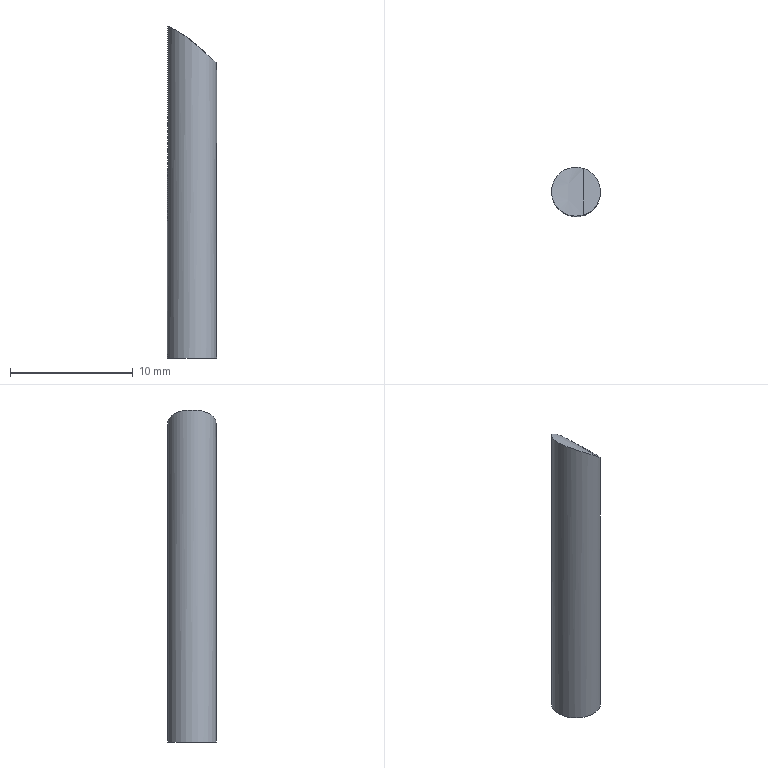Part | NX | features solid 2 | 1 solid | 4 faces | box 4 x 4.001 x 27.078 mm | volume 323.75 mm3 | spline 2 | cylinder 1 | plane 1 | commonest cylinder face diameters 4 x1
STEP:
#1=CARTESIAN_POINT('',(870.5,-198.,17.));
#2=VERTEX_POINT('',#1);
#3=CARTESIAN_POINT('',(872.5,-198.,17.));
#4=DIRECTION('',(0.,0.,-1.));
#5=DIRECTION('',(-1.,0.,0.));
#6=AXIS2_PLACEMENT_3D('',#3,#4,#5);
#7=CIRCLE('',#6,2.);
#8=EDGE_CURVE('',#2,#2,#7,.T.);
#9=ORIENTED_EDGE('',*,*,#8,.F.);
#10=EDGE_LOOP('',(#9));
#11=FACE_BOUND('',#10,.T.);
#12=CARTESIAN_POINT('',(873.077,-199.915,42.346));
#13=VERTEX_POINT('',#12);
#14=CARTESIAN_POINT('',(873.122,-196.099,42.33));
#15=VERTEX_POINT('',#14);
#16=CARTESIAN_POINT('',(873.077,-199.915,42.346));
#17=CARTESIAN_POINT('',(873.426,-199.81,42.025));
#18=CARTESIAN_POINT('',(874.098,-199.426,41.407));
#19=CARTESIAN_POINT('',(874.692,-198.034,40.865));
#20=CARTESIAN_POINT('',(874.135,-196.613,41.387));
#21=CARTESIAN_POINT('',(873.469,-196.212,42.007));
#22=CARTESIAN_POINT('',(873.122,-196.099,42.33));
#23=B_SPLINE_CURVE_WITH_KNOTS('',3,(#16,#17,#18,#19,#20,#21,#22),.UNSPECIFIED.,.F.,.F.,(4,1,1,1,4),(0.00009288,0.001538,0.002982,0.004427,0.005872),.UNSPECIFIED.);
#24=EDGE_CURVE('',#13,#15,#23,.T.);
#25=ORIENTED_EDGE('',*,*,#24,.F.);
#26=CARTESIAN_POINT('',(873.077,-199.915,42.346));
#27=CARTESIAN_POINT('',(872.568,-200.068,42.816));
#28=CARTESIAN_POINT('',(871.655,-200.006,43.483));
#29=CARTESIAN_POINT('',(870.685,-199.041,43.992));
#30=CARTESIAN_POINT('',(870.403,-197.978,44.121));
#31=CARTESIAN_POINT('',(870.707,-196.923,43.989));
#32=CARTESIAN_POINT('',(871.699,-195.974,43.474));
#33=CARTESIAN_POINT('',(872.616,-195.934,42.8));
#34=CARTESIAN_POINT('',(873.122,-196.099,42.33));
#35=B_SPLINE_CURVE_WITH_KNOTS('',3,(#26,#27,#28,#29,#30,#31,#32,#33,#34),.UNSPECIFIED.,.F.,.F.,(4,1,1,1,1,1,4),(0.,0.002104,0.003155,0.004207,0.005259,0.006311,0.008415),.UNSPECIFIED.);
#36=EDGE_CURVE('',#13,#15,#35,.T.);
#37=ORIENTED_EDGE('',*,*,#36,.T.);
#38=EDGE_LOOP('',(#25,#37));
#39=FACE_BOUND('',#38,.T.);
#40=CARTESIAN_POINT('',(872.5,-198.,47.));
#41=DIRECTION('',(0.,0.,-1.));
#42=DIRECTION('',(1.,0.,0.));
#43=AXIS2_PLACEMENT_3D('',#40,#41,#42);
#44=CYLINDRICAL_SURFACE('',#43,2.);
#45=ADVANCED_FACE('',(#11,#39),#44,.T.);
#46=ORIENTED_EDGE('',*,*,#8,.T.);
#47=EDGE_LOOP('',(#46));
#48=FACE_BOUND('',#47,.T.);
#49=CARTESIAN_POINT('',(872.5,-198.,17.));
#50=DIRECTION('',(0.,0.,-1.));
#51=DIRECTION('',(1.,0.,0.));
#52=AXIS2_PLACEMENT_3D('',#49,#50,#51);
#53=PLANE('',#52);
#54=ADVANCED_FACE('',(#48),#53,.T.);
#55=ORIENTED_EDGE('',*,*,#24,.T.);
#56=CARTESIAN_POINT('',(873.077,-199.915,42.346));
#57=CARTESIAN_POINT('',(873.092,-198.64,42.341));
#58=CARTESIAN_POINT('',(873.107,-197.368,42.335));
#59=CARTESIAN_POINT('',(873.122,-196.099,42.33));
#60=B_SPLINE_CURVE_WITH_KNOTS('',3,(#56,#57,#58,#59),.UNSPECIFIED.,.F.,.F.,(4,4),(0.5031,0.6653),.UNSPECIFIED.);
#61=EDGE_CURVE('',#13,#15,#60,.T.);
#62=ORIENTED_EDGE('',*,*,#61,.F.);
#63=EDGE_LOOP('',(#55,#62));
#64=FACE_BOUND('',#63,.T.);
#65=CARTESIAN_POINT('',(874.524,-195.524,41.032));
#66=CARTESIAN_POINT('',(873.095,-196.086,42.354));
#67=CARTESIAN_POINT('',(874.517,-196.774,41.032));
#68=CARTESIAN_POINT('',(873.086,-197.386,42.354));
#69=CARTESIAN_POINT('',(874.511,-198.023,41.032));
#70=CARTESIAN_POINT('',(873.077,-198.686,42.354));
#71=CARTESIAN_POINT('',(874.505,-199.273,41.032));
#72=CARTESIAN_POINT('',(873.068,-199.986,42.354));
#73=B_SPLINE_SURFACE_WITH_KNOTS('',3,1,((#65,#66),(#67,#68),(#69,#70),(#71,#72)),.RULED_SURF.,.F.,.F.,.F.,(4,4),(2,2),(0.4314,0.4981),(0.5388,0.6713),.PIECEWISE_BEZIER_KNOTS.);
#74=ADVANCED_FACE('',(#64),#73,.F.);
#75=ORIENTED_EDGE('',*,*,#61,.T.);
#76=ORIENTED_EDGE('',*,*,#36,.F.);
#77=EDGE_LOOP('',(#75,#76));
#78=FACE_BOUND('',#77,.T.);
#79=CARTESIAN_POINT('',(873.076,-200.043,42.347));
#80=CARTESIAN_POINT('',(871.903,-200.039,43.43));
#81=CARTESIAN_POINT('',(870.451,-200.03,44.094));
#82=CARTESIAN_POINT('',(873.092,-198.684,42.341));
#83=CARTESIAN_POINT('',(871.918,-198.68,43.426));
#84=CARTESIAN_POINT('',(870.465,-198.67,44.092));
#85=CARTESIAN_POINT('',(873.107,-197.325,42.335));
#86=CARTESIAN_POINT('',(871.934,-197.321,43.423));
#87=CARTESIAN_POINT('',(870.479,-197.311,44.09));
#88=CARTESIAN_POINT('',(873.123,-195.966,42.329));
#89=CARTESIAN_POINT('',(871.949,-195.962,43.419));
#90=CARTESIAN_POINT('',(870.493,-195.952,44.088));
#91=(BOUNDED_SURFACE()B_SPLINE_SURFACE(3,2,((#79,#80,#81),(#82,#83,#84),(#85,#86,#87),(#88,#89,#90)),.UNSPECIFIED.,.F.,.F.,.F.)B_SPLINE_SURFACE_WITH_KNOTS((4,4),(3,3),(0.538,0.668),(0.,0.4255),.PIECEWISE_BEZIER_KNOTS.)GEOMETRIC_REPRESENTATION_ITEM()RATIONAL_B_SPLINE_SURFACE(((1.,0.9708,0.9664),(1.,0.9707,0.9663),(1.,0.9706,0.9663),(1.,0.9706,0.9662)))REPRESENTATION_ITEM('')SURFACE());
#92=ADVANCED_FACE('',(#78),#91,.T.);
#93=CLOSED_SHELL('',(#45,#54,#74,#92));
#94=MANIFOLD_SOLID_BREP('',#93);
#95=(LENGTH_UNIT()NAMED_UNIT(*)SI_UNIT(.MILLI.,.METRE.));
#96=UNCERTAINTY_MEASURE_WITH_UNIT(LENGTH_MEASURE(0.0508),#95,'','');
#97=(NAMED_UNIT(*)PLANE_ANGLE_UNIT()SI_UNIT($,.RADIAN.));
#98=(NAMED_UNIT(*)SI_UNIT($,.STERADIAN.)SOLID_ANGLE_UNIT());
#99=(GEOMETRIC_REPRESENTATION_CONTEXT(3)GLOBAL_UNCERTAINTY_ASSIGNED_CONTEXT((#96))GLOBAL_UNIT_ASSIGNED_CONTEXT((#95,#97,#98))REPRESENTATION_CONTEXT('',''));
#100=ADVANCED_BREP_SHAPE_REPRESENTATION('',(#94),#99);